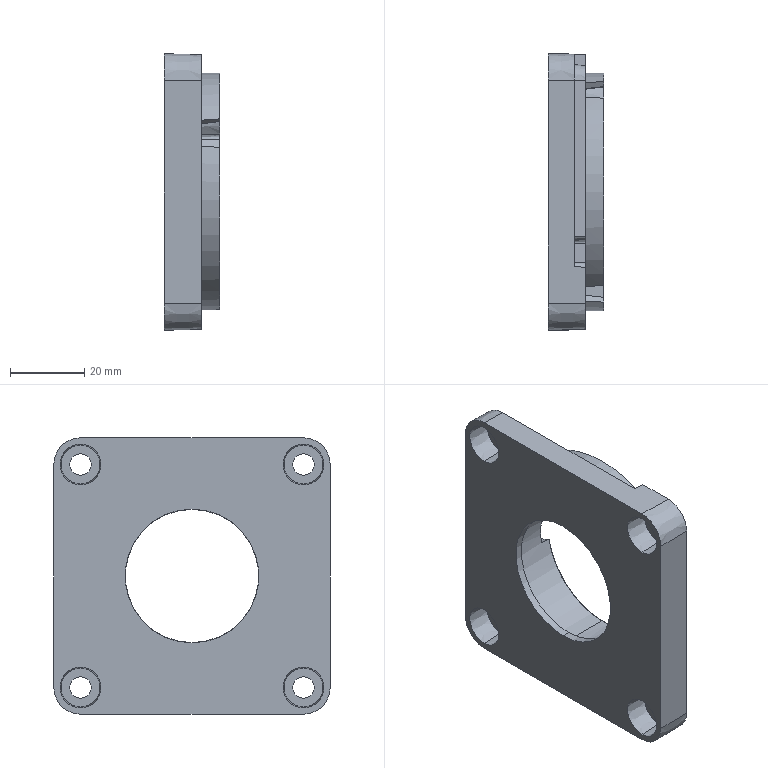Part | SolidWorks | features BaseBody 1 | 1 solid | 141 faces | box 15 x 74.349 x 74.349 mm | volume 38414 mm3 | cone 61 | plane 40 | spline 28 | cylinder 12 | commonest cylinder face diameters 3.3 x6 63.95 x4 41.05 x2